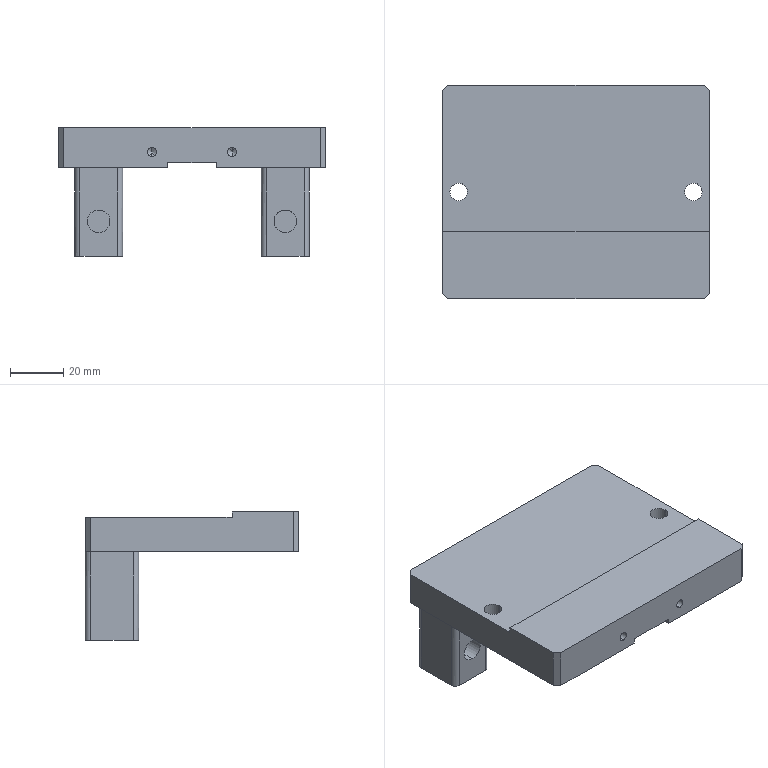NC program | NX | posted with a generic post | part box 100 x 80 x 48 mm
Whole program:
N10 G17 G21 G94 G90
(FLOOR_WALL_1_COPY_COPY_1_COPY_COPY_1 , TOOL : D10JING)
N12 T14 M6
N14 G54
N16 G17 G0 G90 X-28.954 Y46.5 S9500 M3
N18 G43 Z30. H14
N20 Z-16.45
N22 G94 G1 Z-17.95 F1200.
N24 X-28.464 Y45.536
N26 G3 X-27.626 Y44.99 R1.
N28 G2 X-21. Y38. R7.
N30 G1 Y22.
N32 G2 X-28. Y15. R7.
N34 G1 X-42.
N36 G2 X-49. Y22. R7.
N38 G1 Y38.
N40 G2 X-42.374 Y44.99 R7.
N42 G3 X-41.536 Y45.536 R1.
N44 G1 X-41.046 Y46.5
N46 Z-16.45
N48 G0 X-28.954 Z-31.4
N50 G1 Z-32.9
N52 X-28.464 Y45.536
N54 G3 X-27.626 Y44.99 R1.
N56 G2 X-21. Y38. R7.
N58 G1 Y22.
N60 G2 X-28. Y15. R7.
N62 G1 X-42.
N64 G2 X-49. Y22. R7.
N66 G1 Y38.
N68 G2 X-42.374 Y44.99 R7.
N70 G3 X-41.536 Y45.536 R1.
N72 G1 X-41.046 Y46.5
N74 Z-31.4
N76 G0 Z30.
N78 X41.046
N80 Z-16.45
N82 G1 Z-17.95
N84 X41.536 Y45.536
N86 G3 X42.374 Y44.99 R1.
N88 G2 X49. Y38. R7.
N90 G1 Y22.
N92 G2 X42. Y15. R7.
N94 G1 X28.
N96 G2 X21. Y22. R7.
N98 G1 Y38.
N100 G2 X27.626 Y44.99 R7.
N102 G3 X28.464 Y45.536 R1.
N104 G1 X28.954 Y46.5
N106 Z-16.45
N108 G0 X41.046 Z-31.4
N110 G1 Z-32.9
N112 X41.536 Y45.536
N114 G3 X42.374 Y44.99 R1.
N116 G2 X49. Y38. R7.
N118 G1 Y22.
N120 G2 X42. Y15. R7.
N122 G1 X28.
N124 G2 X21. Y22. R7.
N126 G1 Y38.
N128 G2 X27.626 Y44.99 R7.
N130 G3 X28.464 Y45.536 R1.
N132 G1 X28.954 Y46.5
N134 Z-31.4
N136 G0 Z30.
(FLOOR_WALL_1_COPY_COPY_1_COPY , TOOL : D10JING)
N138 X-55.979 Y-41.214
N140 Z-31.5
N142 G1 Z-33.
N144 X-55.5 Y-40.937
N146 G3 X-55. Y-40.071 R1.
N148 G1 Y40.071
N150 X-50.333 Y44.738
N152 Y-44.738
N154 X-50.071 Y-45.
N156 X-45.667
N158 Y15.457
N160 G3 X-42. Y14.5 R7.5
N162 G1 X-41.
N164 Y-45.
N166 X-36.333
N168 Y14.5
N170 X-31.667
N172 Y-45.
N174 X-27.
N176 Y14.567
N178 G3 X-22.333 Y17.087 R7.5
N180 G1 Y-45.
N182 G2 X-22.833 Y-45.866 R1.
N184 G1 X-23.931 Y-46.5
N186 Z-31.5
N188 G0 Z30.
N190 X-46.667 Y46.5
N192 Z-31.5
N194 G1 Z-33.
N196 Y44.555
N198 G3 X-45.667 Y44.543 R1.
N200 G1 Y45.
N202 G3 X-46.167 Y45.866 R1.
N204 G1 X-47.265 Y46.5
N206 Z-31.5
N208 G0 X-23.931
N210 G1 Z-33.
N212 X-22.833 Y45.866
N214 G2 X-22.333 Y45. R1.
N216 G1 Y42.913
N218 Z-31.5
N220 G0 Z30.
N222 X-19.265 Y-46.5
N224 Z-31.5
N226 G1 Z-33.
N228 X-18.167 Y-45.866
N230 G3 X-17.667 Y-45. R1.
N232 G1 Y45.
N234 X-13.
N236 Y-45.
N238 G2 X-13.5 Y-45.866 R1.
N240 G1 X-14.598 Y-46.5
N242 Z-31.5
N244 G0 Z30.
N246 X-28.954 Y46.5
N248 Z-31.5
N250 G1 Z-33.
N252 X-28.464 Y45.536
N254 G3 X-27.626 Y44.99 R1.
N256 G2 X-21. Y38. R7.
N258 G1 Y22.
N260 G2 X-28. Y15. R7.
N262 G1 X-42.
N264 G2 X-49. Y22. R7.
N266 G1 Y38.
N268 G2 X-42.374 Y44.99 R7.
N270 G3 X-41.536 Y45.536 R1.
N272 G1 X-41.046 Y46.5
N274 Z-31.5
N276 G0 Z30.
N278 X3.025 Y-46.14
N280 Z-31.5
N282 G1 Z-33.
N284 X3.5 Y-45.866
N286 G3 X4. Y-45. R1.
N288 G1 Y45.
N290 X8.667
N292 Y-45.
N294 X13.333
N296 Y45.
N298 X18.
N300 Y-45.
N302 X22.667
N304 Y16.727
N306 G3 X27.333 Y14.53 R7.5
N308 G1 Y-45.
N310 X32.
N312 Y14.5
N314 X36.667
N316 Y-45.
N318 X41.333
N320 Y14.5
N322 X42.
N324 G3 X46. Y15.656 R7.5
N326 G1 Y-45.
N328 G2 X45.5 Y-45.866 R1.
N330 G1 X44.402 Y-46.5
N332 Z-31.5
N334 G0 Z30.
N336 X21.702 Y46.5
N338 Z-31.5
N340 G1 Z-33.
N342 Y43.009
N344 G3 X22.667 Y43.273 R1.
N346 G1 Y45.
N348 G3 X22.167 Y45.866 R1.
N350 G1 X21.069 Y46.5
N352 Z-31.5
N354 G0 X44.402
N356 G1 Z-33.
N358 X45.5 Y45.866
N360 G2 X46. Y45. R1.
N362 G1 Y44.344
N364 Z-31.5
N366 G0 Z30.
N368 X48.037 Y-46.5
N370 Z-31.5
N372 G1 Z-33.
N374 X50.167 Y-45.27
N376 G3 X50.667 Y-44.404 R1.
N378 G1 Y44.404
N380 G3 X50.167 Y45.27 R1.
N382 G1 X48.037 Y46.5
N384 Z-31.5
N386 G0 X41.046
N388 G1 Z-33.
N390 X41.536 Y45.536
N392 G3 X42.374 Y44.99 R1.
N394 G2 X49. Y38. R7.
N396 G1 Y22.
N398 G2 X42. Y15. R7.
N400 G1 X28.
N402 G2 X21. Y22. R7.
N404 G1 Y38.
N406 G2 X27.626 Y44.99 R7.
N408 G3 X28.464 Y45.536 R1.
N410 G1 X28.954 Y46.5
N412 Z-31.5
N414 G0 Z30.
(FLOOR_WALL_1_COPY_COPY_1_COPY_COPY , TOOL : D10JING)
N416 X-2.4 Y-46.5
N418 Z-33.5
N420 G1 Z-35.
N422 X-2.899 Y-44.134
N424 G3 X-3.399 Y-45. R1.
N426 G1 Y45.
N428 X0.
N430 Y-45.
N432 X3.4
N434 Y45.
N436 G3 X2.9 Y45.866 R1.
N438 G1 X1.802 Y46.5
N440 Z-33.5
N442 G0 X-2.302
N444 G1 Z-35.
N446 X-3.4 Y45.866
N448 G3 X-3.9 Y45. R1.
N450 G1 Y-45.
N452 G3 X-3.4 Y-45.866 R1.
N454 G1 X3.4
N456 G3 X3.9 Y-45. R1.
N458 G1 Y45.
N460 G3 X3.4 Y45.866 R1.
N462 G1 X2.302 Y46.5
N464 Z-33.5
N466 G0 Z30.
N468 M5
(HOLE_MILLING , TOOL : D6)
N470 T12 M6
N472 G54
N474 G17 G0 G90 X-44. Y0. S9500 M3
N476 G43 Z30. H12
N478 Z-32.5
N480 G94 G3 X-45.25 Y1.25 R1.25 F1500.
N482 X-46.5 Y0. R1.25
N484 X-46.5 Y0. Z-33.1 I2.5 J0.
N486 X-46.5 Y0. Z-33.7 I2.5 J0.
N488 X-46.5 Y0. Z-34.3 I2.5 J0.
N490 X-46.5 Y0. Z-34.9 I2.5 J0.
N492 X-46.5 Y0. Z-35.5 I2.5 J0.
N494 X-46.5 Y0. Z-36.1 I2.5 J0.
N496 X-46.5 Y0. Z-36.7 I2.5 J0.
N498 X-46.5 Y0. Z-37.3 I2.5 J0.
N500 X-46.5 Y0. Z-37.9 I2.5 J0.
N502 X-46.5 Y0. Z-38.5 I2.5 J0.
N504 X-46.5 Y0. Z-39.1 I2.5 J0.
N506 X-46.5 Y0. Z-39.7 I2.5 J0.
N508 X-45.25 Y-2.165 Z-39.8 R2.5
N510 X-41.835 Y-1.25 R2.5
N512 X-45.25 Y-2.165 R-2.5
N514 X-43.542 Y-1.708 R1.25
N516 X-44. Y0. R1.25
N518 G0 Z30.
N520 X44.
N522 Z-32.5
N524 G3 X42.75 Y1.25 R1.25
N526 X41.5 Y0. R1.25
N528 X41.5 Y0. Z-33.1 I2.5 J0.
N530 X41.5 Y0. Z-33.7 I2.5 J0.
N532 X41.5 Y0. Z-34.3 I2.5 J0.
N534 X41.5 Y0. Z-34.9 I2.5 J0.
N536 X41.5 Y0. Z-35.5 I2.5 J0.
N538 X41.5 Y0. Z-36.1 I2.5 J0.
N540 X41.5 Y0. Z-36.7 I2.5 J0.
N542 X41.5 Y0. Z-37.3 I2.5 J0.
N544 X41.5 Y0. Z-37.9 I2.5 J0.
N546 X41.5 Y0. Z-38.5 I2.5 J0.
N548 X41.5 Y0. Z-39.1 I2.5 J0.
N550 X41.5 Y0. Z-39.7 I2.5 J0.
N552 X42.75 Y-2.165 Z-39.8 R2.5
N554 X46.165 Y-1.25 R2.5
N556 X42.75 Y-2.165 R-2.5
N558 X44.458 Y-1.708 R1.25
N560 X44. Y0. R1.25
N562 G0 Z30.
N564 M5
(DRILLING , TOOL : D6A45)
N566 T01 M6
N568 G54
N570 G17 G0 G90 X-44. Y0. S9500 M3
N572 G43 Z30. H1
N574 G94 G81 G98 Z-34. F250. R-30.
N576 X0. Y30. Z-36. R-32.
N578 Y0.
N580 Y-30.
N582 X44. Y0. Z-34. R-30.
N584 G80
N586 G0 X44. Y0. Z30.
N588 M5
(DRILLING_COPY_COPY , TOOL : 6.6ZT)
N590 T09 M6
N592 G54
N594 G17 G0 G90 X-44. Y0. S2000 M3
N596 G43 Z30. H9
N598 G94 G83 G98 Z-49.483 F300. Q2. R-30.
N600 X44.
N602 G80
N604 G0 X44. Y0. Z30.
N606 M5
(DRILLING_COPY_COPY_COPY , TOOL : 2.5ZT)
N608 T02 M6
N610 G54
N612 G17 G0 G90 X0. Y30. S2000 M3
N614 G43 Z30. H2
N616 G94 G83 G98 Z-43.251 F100. Q2. R-32.
N618 Y0.
N620 Y-30.
N622 G80
N624 G0 X0. Y-30. Z30.
N626 M5
(PLANAR_MILL_COPY_COPY_COPY , TOOL : D6A45)
N628 T01 M6
N630 G54
N632 G17 G0 G90 X-47.069 Y1.461 S9500 M3
N634 G43 Z30. H1
N636 Z-32.5
N638 G94 G1 Z-34. F1250.
N640 X-48.1 Y0.866
N642 G3 X-48.6 Y0. R1.
N644 X-46.09 Y-4.092 R4.591
N646 X-41.293 Y-3.72 R4.618
N648 X-39.9 Y-2.091 R4.545
N650 X-39.9 Y2.091 R4.623
N652 X-41.293 Y3.72 R4.545
N654 X-46.09 Y4.092 R4.618
N656 X-48.6 Y0. R4.591
N658 X-48.1 Y-0.866 R1.
N660 G1 X-47.069 Y-1.461
N662 Z-32.5
N664 G0 Z30.
N666 X-23.037 Y42.5
N668 Z-32.5
N670 G1 Z-34.
N672 X-23.358 Y41.899
N674 G3 X-23.327 Y40.9 R1.
N676 G1 X-9.1
N678 G2 X-8.1 Y39.9 R1.
N680 G1 Y-39.9
N682 G2 X-9.1 Y-40.9 R1.
N684 G1 X-47.959
N686 G2 X-48.666 Y-40.607 R1.
N688 G1 X-50.607 Y-38.666
N690 G2 X-50.9 Y-37.959 R1.
N692 G1 Y37.959
N694 G2 X-50.607 Y38.666 R1.
N696 G1 X-48.666 Y40.607
N698 G2 X-47.959 Y40.9 R1.
N700 G1 X-46.673
N702 G3 X-46.642 Y41.899 R1.
N704 G1 X-46.963 Y42.5
N706 Z-32.5
N708 G0 Z30.
N710 X46.963
N712 Z-32.5
N714 G1 Z-34.
N716 X46.642 Y41.899
N718 G3 X46.673 Y40.9 R1.
N720 G1 X47.959
N722 G2 X48.666 Y40.607 R1.
N724 G1 X50.607 Y38.666
N726 G2 X50.9 Y37.959 R1.
N728 G1 Y-37.959
N730 G2 X50.607 Y-38.666 R1.
N732 G1 X48.666 Y-40.607
N734 G2 X47.959 Y-40.9 R1.
N736 G1 X9.1
N738 G2 X8.1 Y-39.9 R1.
N740 G1 Y39.9
N742 G2 X9.1 Y40.9 R1.
N744 G1 X23.327
N746 G3 X23.358 Y41.899 R1.
N748 G1 X23.037 Y42.5
N750 Z-32.5
N752 G0 Z30.
N754 X47.069 Y-1.461
N756 Z-32.5
N758 G1 Z-34.
N760 X48.1 Y-0.866
N762 G3 X48.6 Y0. R1.
N764 X46.09 Y4.092 R4.591
N766 X41.293 Y3.72 R4.618
N768 X39.9 Y2.091 R4.545
N770 X39.9 Y-2.091 R4.623
N772 X41.293 Y-3.72 R4.545
N774 X46.09 Y-4.092 R4.618
N776 X48.6 Y0. R4.591
N778 X48.1 Y0.866 R1.
N780 G1 X47.069 Y1.461
N782 Z-32.5
N784 G0 Z30.
N786 M5
(FLOOR_WALL_1_COPY_COPY_1_COPY_COPY_COPY , TOOL : D6)
N788 T12 M6
N790 G54
N792 G17 G0 G90 X4.356 Y-44.247 S9500 M3
N794 G43 Z30. H12
N796 Z-33.5
N798 G94 G1 Z-35. F1200.
N800 G41 X4.45 Y-44.212 D12
N802 X5.65 Y-43.52
N804 G3 X5.95 Y-43. R0.6
N806 G1 Y43.
N808 G3 X5.65 Y43.52 R0.6
N810 G1 X4.45 Y44.212
N812 G40
N814 X4.356 Y44.247
N816 Z-33.5
N818 G0 X-4.356
N820 G1 Z-35.
N822 G41 X-4.45 Y44.212
N824 X-5.65 Y43.52
N826 G3 X-5.95 Y43. R0.6
N828 G1 Y-43.
N830 G3 X-5.65 Y-43.52 R0.6
N832 G1 X-4.45 Y-44.212
N834 G40
N836 X-4.356 Y-44.247
N838 Z-33.5
N840 G0 Z30.
N842 M5
N844 M2